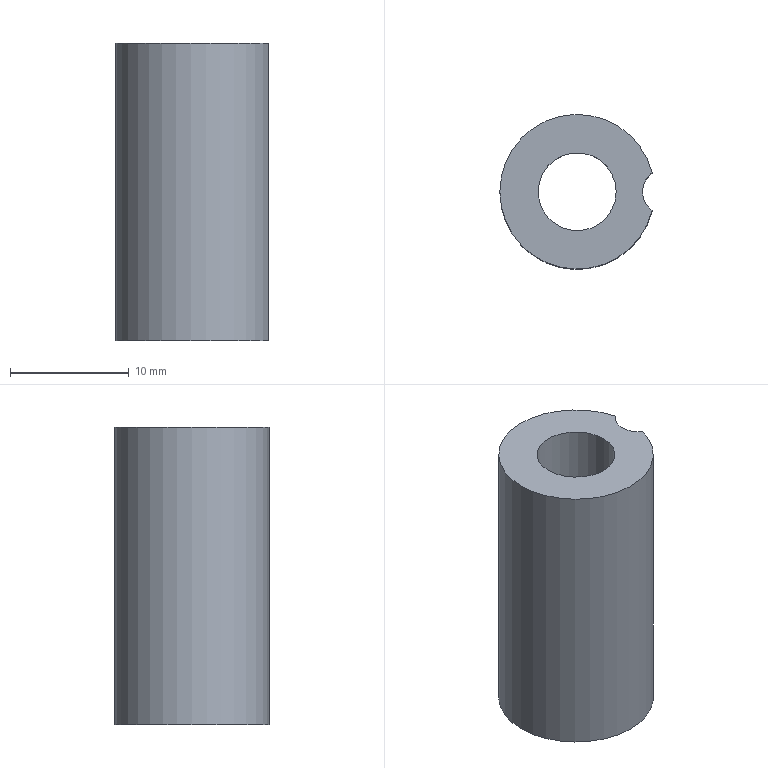Part | NX | features solid 2 | 1 solid | 7 faces | box 12.8 x 13 x 25 mm | volume 2050 mm3 | cylinder 4 | plane 3 | commonest cylinder face diameters 4 x1 6.56 x1 8.4 x1 13 x1
STEP:
#1=CARTESIAN_POINT('',(-93.7,-264.52,-49.));
#2=VERTEX_POINT('',#1);
#3=CARTESIAN_POINT('',(-93.7,-267.72,-49.));
#4=VERTEX_POINT('',#3);
#5=CARTESIAN_POINT('',(-92.5,-266.12,-49.));
#6=DIRECTION('',(0.,0.,1.));
#7=DIRECTION('',(1.,0.,0.));
#8=AXIS2_PLACEMENT_3D('',#5,#6,#7);
#9=CIRCLE('',#8,2.);
#10=EDGE_CURVE('',#2,#4,#9,.T.);
#11=ORIENTED_EDGE('',*,*,#10,.T.);
#12=CARTESIAN_POINT('',(-93.7,-267.72,-74.));
#13=VERTEX_POINT('',#12);
#14=CARTESIAN_POINT('',(-93.7,-267.72,-74.));
#15=DIRECTION('',(0.,0.,1.));
#16=VECTOR('',#15,1000.);
#17=LINE('',#14,#16);
#18=EDGE_CURVE('',#13,#4,#17,.T.);
#19=ORIENTED_EDGE('',*,*,#18,.F.);
#20=CARTESIAN_POINT('',(-93.7,-264.52,-74.));
#21=VERTEX_POINT('',#20);
#22=CARTESIAN_POINT('',(-92.5,-266.12,-74.));
#23=DIRECTION('',(0.,0.,1.));
#24=DIRECTION('',(1.,0.,0.));
#25=AXIS2_PLACEMENT_3D('',#22,#23,#24);
#26=CIRCLE('',#25,2.);
#27=EDGE_CURVE('',#21,#13,#26,.T.);
#28=ORIENTED_EDGE('',*,*,#27,.F.);
#29=CARTESIAN_POINT('',(-93.7,-264.52,-74.));
#30=DIRECTION('',(0.,0.,1.));
#31=VECTOR('',#30,1000.);
#32=LINE('',#29,#31);
#33=EDGE_CURVE('',#2,#21,#32,.F.);
#34=ORIENTED_EDGE('',*,*,#33,.F.);
#35=EDGE_LOOP('',(#11,#19,#28,#34));
#36=FACE_BOUND('',#35,.T.);
#37=CARTESIAN_POINT('',(-92.5,-266.12,-74.));
#38=DIRECTION('',(0.,0.,1.));
#39=DIRECTION('',(1.,0.,0.));
#40=AXIS2_PLACEMENT_3D('',#37,#38,#39);
#41=CYLINDRICAL_SURFACE('',#40,2.);
#42=ADVANCED_FACE('',(#36),#41,.F.);
#43=CARTESIAN_POINT('',(-100.,-266.12,-49.));
#44=DIRECTION('',(0.,0.,1.));
#45=DIRECTION('',(1.,0.,0.));
#46=AXIS2_PLACEMENT_3D('',#43,#44,#45);
#47=CIRCLE('',#46,6.5);
#48=EDGE_CURVE('',#2,#4,#47,.T.);
#49=ORIENTED_EDGE('',*,*,#48,.F.);
#50=ORIENTED_EDGE('',*,*,#33,.T.);
#51=CARTESIAN_POINT('',(-100.,-266.12,-74.));
#52=DIRECTION('',(0.,0.,1.));
#53=DIRECTION('',(1.,0.,0.));
#54=AXIS2_PLACEMENT_3D('',#51,#52,#53);
#55=CIRCLE('',#54,6.5);
#56=EDGE_CURVE('',#21,#13,#55,.T.);
#57=ORIENTED_EDGE('',*,*,#56,.T.);
#58=ORIENTED_EDGE('',*,*,#18,.T.);
#59=EDGE_LOOP('',(#49,#50,#57,#58));
#60=FACE_BOUND('',#59,.T.);
#61=CARTESIAN_POINT('',(-100.,-266.12,-74.));
#62=DIRECTION('',(0.,0.,1.));
#63=DIRECTION('',(1.,0.,0.));
#64=AXIS2_PLACEMENT_3D('',#61,#62,#63);
#65=CYLINDRICAL_SURFACE('',#64,6.5);
#66=ADVANCED_FACE('',(#60),#65,.T.);
#67=CARTESIAN_POINT('',(-95.8,-266.12,-74.));
#68=VERTEX_POINT('',#67);
#69=CARTESIAN_POINT('',(-100.,-266.12,-74.));
#70=DIRECTION('',(0.,0.,1.));
#71=DIRECTION('',(1.,0.,0.));
#72=AXIS2_PLACEMENT_3D('',#69,#70,#71);
#73=CIRCLE('',#72,4.2);
#74=EDGE_CURVE('',#68,#68,#73,.T.);
#75=ORIENTED_EDGE('',*,*,#74,.T.);
#76=EDGE_LOOP('',(#75));
#77=FACE_BOUND('',#76,.T.);
#78=ORIENTED_EDGE('',*,*,#27,.T.);
#79=ORIENTED_EDGE('',*,*,#56,.F.);
#80=EDGE_LOOP('',(#78,#79));
#81=FACE_BOUND('',#80,.T.);
#82=CARTESIAN_POINT('',(-92.,-266.12,-74.));
#83=DIRECTION('',(0.,0.,1.));
#84=DIRECTION('',(1.,0.,0.));
#85=AXIS2_PLACEMENT_3D('',#82,#83,#84);
#86=PLANE('',#85);
#87=ADVANCED_FACE('',(#77,#81),#86,.F.);
#88=CARTESIAN_POINT('',(-96.72,-266.12,-49.));
#89=VERTEX_POINT('',#88);
#90=CARTESIAN_POINT('',(-100.,-266.12,-49.));
#91=DIRECTION('',(0.,0.,1.));
#92=DIRECTION('',(1.,0.,0.));
#93=AXIS2_PLACEMENT_3D('',#90,#91,#92);
#94=CIRCLE('',#93,3.28);
#95=EDGE_CURVE('',#89,#89,#94,.T.);
#96=ORIENTED_EDGE('',*,*,#95,.F.);
#97=EDGE_LOOP('',(#96));
#98=FACE_BOUND('',#97,.T.);
#99=ORIENTED_EDGE('',*,*,#10,.F.);
#100=ORIENTED_EDGE('',*,*,#48,.T.);
#101=EDGE_LOOP('',(#99,#100));
#102=FACE_BOUND('',#101,.T.);
#103=CARTESIAN_POINT('',(-92.,-266.12,-49.));
#104=DIRECTION('',(0.,0.,1.));
#105=DIRECTION('',(1.,0.,0.));
#106=AXIS2_PLACEMENT_3D('',#103,#104,#105);
#107=PLANE('',#106);
#108=ADVANCED_FACE('',(#98,#102),#107,.T.);
#109=CARTESIAN_POINT('',(-96.72,-266.12,-57.));
#110=VERTEX_POINT('',#109);
#111=CARTESIAN_POINT('',(-100.,-266.12,-57.));
#112=DIRECTION('',(0.,0.,1.));
#113=DIRECTION('',(1.,0.,0.));
#114=AXIS2_PLACEMENT_3D('',#111,#112,#113);
#115=CIRCLE('',#114,3.28);
#116=EDGE_CURVE('',#110,#110,#115,.F.);
#117=ORIENTED_EDGE('',*,*,#116,.T.);
#118=EDGE_LOOP('',(#117));
#119=FACE_BOUND('',#118,.T.);
#120=ORIENTED_EDGE('',*,*,#95,.T.);
#121=EDGE_LOOP('',(#120));
#122=FACE_BOUND('',#121,.T.);
#123=CARTESIAN_POINT('',(-100.,-266.12,-57.));
#124=DIRECTION('',(0.,0.,1.));
#125=DIRECTION('',(1.,0.,0.));
#126=AXIS2_PLACEMENT_3D('',#123,#124,#125);
#127=CYLINDRICAL_SURFACE('',#126,3.28);
#128=ADVANCED_FACE('',(#119,#122),#127,.F.);
#129=CARTESIAN_POINT('',(-95.8,-266.12,-57.));
#130=VERTEX_POINT('',#129);
#131=CARTESIAN_POINT('',(-100.,-266.12,-57.));
#132=DIRECTION('',(0.,0.,1.));
#133=DIRECTION('',(1.,0.,0.));
#134=AXIS2_PLACEMENT_3D('',#131,#132,#133);
#135=CIRCLE('',#134,4.2);
#136=EDGE_CURVE('',#130,#130,#135,.T.);
#137=ORIENTED_EDGE('',*,*,#136,.F.);
#138=EDGE_LOOP('',(#137));
#139=FACE_BOUND('',#138,.T.);
#140=ORIENTED_EDGE('',*,*,#116,.F.);
#141=EDGE_LOOP('',(#140));
#142=FACE_BOUND('',#141,.T.);
#143=CARTESIAN_POINT('',(-100.,-266.12,-57.));
#144=DIRECTION('',(0.,0.,1.));
#145=DIRECTION('',(1.,0.,0.));
#146=AXIS2_PLACEMENT_3D('',#143,#144,#145);
#147=PLANE('',#146);
#148=ADVANCED_FACE('',(#139,#142),#147,.F.);
#149=ORIENTED_EDGE('',*,*,#74,.F.);
#150=EDGE_LOOP('',(#149));
#151=FACE_BOUND('',#150,.T.);
#152=ORIENTED_EDGE('',*,*,#136,.T.);
#153=EDGE_LOOP('',(#152));
#154=FACE_BOUND('',#153,.T.);
#155=CARTESIAN_POINT('',(-100.,-266.12,-74.));
#156=DIRECTION('',(0.,0.,1.));
#157=DIRECTION('',(1.,0.,0.));
#158=AXIS2_PLACEMENT_3D('',#155,#156,#157);
#159=CYLINDRICAL_SURFACE('',#158,4.2);
#160=ADVANCED_FACE('',(#151,#154),#159,.F.);
#161=CLOSED_SHELL('',(#42,#66,#87,#108,#128,#148,#160));
#162=MANIFOLD_SOLID_BREP('',#161);
#163=(LENGTH_UNIT()NAMED_UNIT(*)SI_UNIT(.MILLI.,.METRE.));
#164=UNCERTAINTY_MEASURE_WITH_UNIT(LENGTH_MEASURE(0.00001),#163,'','');
#165=(NAMED_UNIT(*)PLANE_ANGLE_UNIT()SI_UNIT($,.RADIAN.));
#166=(NAMED_UNIT(*)SI_UNIT($,.STERADIAN.)SOLID_ANGLE_UNIT());
#167=(GEOMETRIC_REPRESENTATION_CONTEXT(3)GLOBAL_UNCERTAINTY_ASSIGNED_CONTEXT((#164))GLOBAL_UNIT_ASSIGNED_CONTEXT((#163,#165,#166))REPRESENTATION_CONTEXT('',''));
#168=ADVANCED_BREP_SHAPE_REPRESENTATION('',(#162),#167);